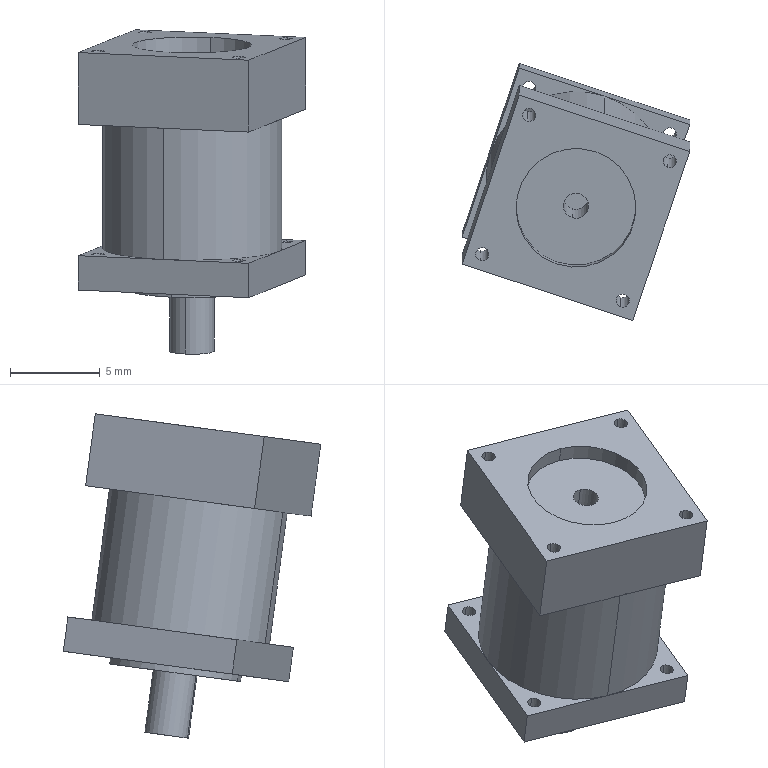Part | SolidWorks | features SplitBody 1 | 1 solid | 51 faces | box 12.695 x 14.369 x 18.106 mm | volume 1159 mm3 | cylinder 28 | plane 23 | commonest cylinder face diameters 0.739 x16 1.408 x2 2.464 x2 6.688 x2 7.04 x2 7.392 x2